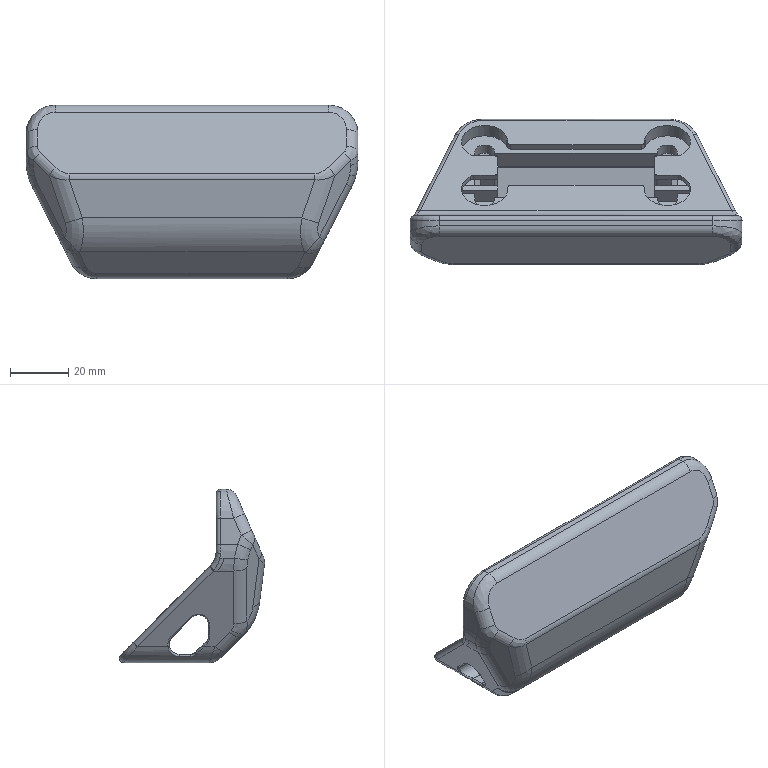Part | SolidWorks | features BaseBody 1 | 1 solid | 297 faces | box 114.193 x 49.996 x 59.691 mm | volume 84846 mm3 | cylinder 135 | plane 112 | spline 44 | torus 4 | cone 2 | commonest cylinder face diameters 12 x14 8 x13 2 x12 10 x12 16 x10 1 x8